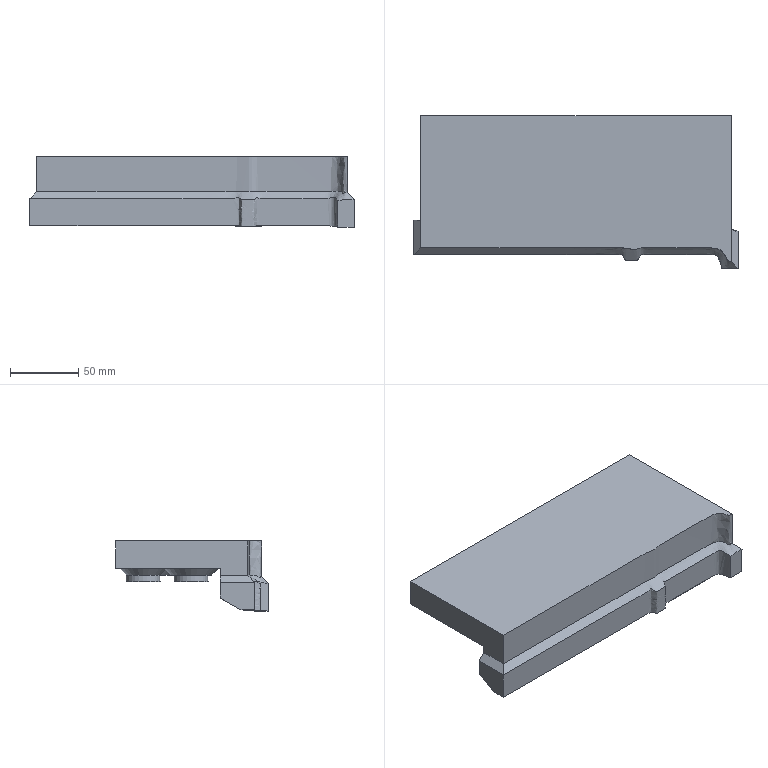Part | NX | features solid 2 | 1 solid | 32 faces | box 236.793 x 111.124 x 51.282 mm | volume 621920 mm3 | plane 15 | spline 10 | cone 5 | cylinder 2 | commonest cylinder face diameters 25 x2